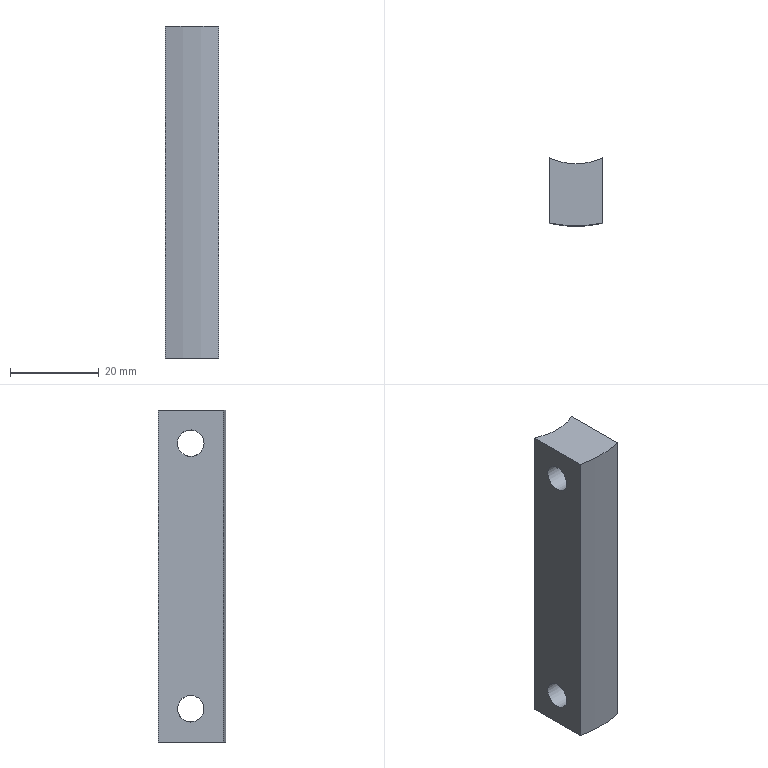Part | NX | features DATUM_CSYS 3, EXTRUDE 2, SKETCH 2 | 1 solid | 8 faces | box 12 x 15.351 x 75 mm | volume 12124 mm3 | plane 4 | cylinder 4 | commonest cylinder face diameters 6 x2 28 x1 56 x1
STEP:
#1=CARTESIAN_POINT('',(-6.,-20.,-27.));
#2=VERTEX_POINT('',#1);
#3=CARTESIAN_POINT('',(-6.,-20.,-30.));
#4=DIRECTION('',(-1.,0.,0.));
#5=DIRECTION('',(0.,0.,1.));
#6=AXIS2_PLACEMENT_3D('',#3,#4,#5);
#7=CIRCLE('',#6,3.);
#8=EDGE_CURVE('',#2,#2,#7,.T.);
#9=ORIENTED_EDGE('',*,*,#8,.F.);
#10=EDGE_LOOP('',(#9));
#11=FACE_BOUND('',#10,.T.);
#12=CARTESIAN_POINT('',(-6.,-20.,27.));
#13=VERTEX_POINT('',#12);
#14=CARTESIAN_POINT('',(-6.,-20.,30.));
#15=DIRECTION('',(-1.,0.,0.));
#16=DIRECTION('',(0.,0.,-1.));
#17=AXIS2_PLACEMENT_3D('',#14,#15,#16);
#18=CIRCLE('',#17,3.);
#19=EDGE_CURVE('',#13,#13,#18,.T.);
#20=ORIENTED_EDGE('',*,*,#19,.F.);
#21=EDGE_LOOP('',(#20));
#22=FACE_BOUND('',#21,.T.);
#23=CARTESIAN_POINT('',(-6.,-12.649,-37.5));
#24=VERTEX_POINT('',#23);
#25=CARTESIAN_POINT('',(-6.,-27.35,-37.5));
#26=VERTEX_POINT('',#25);
#27=CARTESIAN_POINT('',(-6.,-12.649,-37.5));
#28=DIRECTION('',(0.,-1.,0.));
#29=VECTOR('',#28,1000.);
#30=LINE('',#27,#29);
#31=EDGE_CURVE('',#24,#26,#30,.T.);
#32=ORIENTED_EDGE('',*,*,#31,.T.);
#33=CARTESIAN_POINT('',(-6.,-27.35,37.5));
#34=VERTEX_POINT('',#33);
#35=CARTESIAN_POINT('',(-6.,-27.35,37.5));
#36=DIRECTION('',(0.,0.,-1.));
#37=VECTOR('',#36,1000.);
#38=LINE('',#35,#37);
#39=EDGE_CURVE('',#34,#26,#38,.T.);
#40=ORIENTED_EDGE('',*,*,#39,.F.);
#41=CARTESIAN_POINT('',(-6.,-12.649,37.5));
#42=VERTEX_POINT('',#41);
#43=CARTESIAN_POINT('',(-6.,-12.649,37.5));
#44=DIRECTION('',(0.,-1.,0.));
#45=VECTOR('',#44,1000.);
#46=LINE('',#43,#45);
#47=EDGE_CURVE('',#42,#34,#46,.T.);
#48=ORIENTED_EDGE('',*,*,#47,.F.);
#49=CARTESIAN_POINT('',(-6.,-12.649,37.5));
#50=DIRECTION('',(0.,0.,-1.));
#51=VECTOR('',#50,1000.);
#52=LINE('',#49,#51);
#53=EDGE_CURVE('',#42,#24,#52,.T.);
#54=ORIENTED_EDGE('',*,*,#53,.T.);
#55=EDGE_LOOP('',(#32,#40,#48,#54));
#56=FACE_BOUND('',#55,.T.);
#57=CARTESIAN_POINT('',(-6.,-12.649,37.5));
#58=DIRECTION('',(1.,0.,0.));
#59=DIRECTION('',(0.,0.,-1.));
#60=AXIS2_PLACEMENT_3D('',#57,#58,#59);
#61=PLANE('',#60);
#62=ADVANCED_FACE('',(#11,#22,#56),#61,.F.);
#63=CARTESIAN_POINT('',(6.,-27.35,-37.5));
#64=VERTEX_POINT('',#63);
#65=CARTESIAN_POINT('',(-0.000002247,0.,-37.5));
#66=DIRECTION('',(0.,0.,1.));
#67=DIRECTION('',(1.,0.,0.));
#68=AXIS2_PLACEMENT_3D('',#65,#66,#67);
#69=CIRCLE('',#68,28.);
#70=EDGE_CURVE('',#26,#64,#69,.T.);
#71=ORIENTED_EDGE('',*,*,#70,.T.);
#72=CARTESIAN_POINT('',(6.,-27.35,37.5));
#73=VERTEX_POINT('',#72);
#74=CARTESIAN_POINT('',(6.,-27.35,37.5));
#75=DIRECTION('',(0.,0.,-1.));
#76=VECTOR('',#75,1000.);
#77=LINE('',#74,#76);
#78=EDGE_CURVE('',#73,#64,#77,.T.);
#79=ORIENTED_EDGE('',*,*,#78,.F.);
#80=CARTESIAN_POINT('',(-0.000002247,0.,37.5));
#81=DIRECTION('',(0.,0.,1.));
#82=DIRECTION('',(1.,0.,0.));
#83=AXIS2_PLACEMENT_3D('',#80,#81,#82);
#84=CIRCLE('',#83,28.);
#85=EDGE_CURVE('',#34,#73,#84,.T.);
#86=ORIENTED_EDGE('',*,*,#85,.F.);
#87=ORIENTED_EDGE('',*,*,#39,.T.);
#88=EDGE_LOOP('',(#71,#79,#86,#87));
#89=FACE_BOUND('',#88,.T.);
#90=CARTESIAN_POINT('',(-0.000002247,0.,37.5));
#91=DIRECTION('',(0.,0.,-1.));
#92=DIRECTION('',(-1.,0.,0.));
#93=AXIS2_PLACEMENT_3D('',#90,#91,#92);
#94=CYLINDRICAL_SURFACE('',#93,28.);
#95=ADVANCED_FACE('',(#89),#94,.T.);
#96=CARTESIAN_POINT('',(6.,-23.,-30.));
#97=VERTEX_POINT('',#96);
#98=CARTESIAN_POINT('',(6.,-20.,-30.));
#99=DIRECTION('',(-1.,0.,0.));
#100=DIRECTION('',(0.,-1.,0.));
#101=AXIS2_PLACEMENT_3D('',#98,#99,#100);
#102=CIRCLE('',#101,3.);
#103=EDGE_CURVE('',#97,#97,#102,.T.);
#104=ORIENTED_EDGE('',*,*,#103,.T.);
#105=EDGE_LOOP('',(#104));
#106=FACE_BOUND('',#105,.T.);
#107=CARTESIAN_POINT('',(6.,-23.,30.));
#108=VERTEX_POINT('',#107);
#109=CARTESIAN_POINT('',(6.,-20.,30.));
#110=DIRECTION('',(-1.,0.,0.));
#111=DIRECTION('',(0.,-1.,0.));
#112=AXIS2_PLACEMENT_3D('',#109,#110,#111);
#113=CIRCLE('',#112,3.);
#114=EDGE_CURVE('',#108,#108,#113,.T.);
#115=ORIENTED_EDGE('',*,*,#114,.T.);
#116=EDGE_LOOP('',(#115));
#117=FACE_BOUND('',#116,.T.);
#118=CARTESIAN_POINT('',(6.,-12.649,-37.5));
#119=VERTEX_POINT('',#118);
#120=CARTESIAN_POINT('',(6.,-27.35,-37.5));
#121=DIRECTION('',(0.,1.,0.));
#122=VECTOR('',#121,1000.);
#123=LINE('',#120,#122);
#124=EDGE_CURVE('',#64,#119,#123,.T.);
#125=ORIENTED_EDGE('',*,*,#124,.T.);
#126=CARTESIAN_POINT('',(6.,-12.649,37.5));
#127=VERTEX_POINT('',#126);
#128=CARTESIAN_POINT('',(6.,-12.649,37.5));
#129=DIRECTION('',(0.,0.,-1.));
#130=VECTOR('',#129,1000.);
#131=LINE('',#128,#130);
#132=EDGE_CURVE('',#127,#119,#131,.T.);
#133=ORIENTED_EDGE('',*,*,#132,.F.);
#134=CARTESIAN_POINT('',(6.,-27.35,37.5));
#135=DIRECTION('',(0.,1.,0.));
#136=VECTOR('',#135,1000.);
#137=LINE('',#134,#136);
#138=EDGE_CURVE('',#73,#127,#137,.T.);
#139=ORIENTED_EDGE('',*,*,#138,.F.);
#140=ORIENTED_EDGE('',*,*,#78,.T.);
#141=EDGE_LOOP('',(#125,#133,#139,#140));
#142=FACE_BOUND('',#141,.T.);
#143=CARTESIAN_POINT('',(6.,-27.35,37.5));
#144=DIRECTION('',(-1.,0.,0.));
#145=DIRECTION('',(0.,-1.,0.));
#146=AXIS2_PLACEMENT_3D('',#143,#144,#145);
#147=PLANE('',#146);
#148=ADVANCED_FACE('',(#106,#117,#142),#147,.F.);
#149=CARTESIAN_POINT('',(-0.000002247,0.,-37.5));
#150=DIRECTION('',(0.,0.,-1.));
#151=DIRECTION('',(1.,0.,0.));
#152=AXIS2_PLACEMENT_3D('',#149,#150,#151);
#153=CIRCLE('',#152,14.);
#154=EDGE_CURVE('',#119,#24,#153,.T.);
#155=ORIENTED_EDGE('',*,*,#154,.T.);
#156=ORIENTED_EDGE('',*,*,#53,.F.);
#157=CARTESIAN_POINT('',(-0.000002247,0.,37.5));
#158=DIRECTION('',(0.,0.,-1.));
#159=DIRECTION('',(1.,0.,0.));
#160=AXIS2_PLACEMENT_3D('',#157,#158,#159);
#161=CIRCLE('',#160,14.);
#162=EDGE_CURVE('',#127,#42,#161,.T.);
#163=ORIENTED_EDGE('',*,*,#162,.F.);
#164=ORIENTED_EDGE('',*,*,#132,.T.);
#165=EDGE_LOOP('',(#155,#156,#163,#164));
#166=FACE_BOUND('',#165,.T.);
#167=CARTESIAN_POINT('',(-0.000002247,0.,37.5));
#168=DIRECTION('',(0.,0.,-1.));
#169=DIRECTION('',(-1.,0.,0.));
#170=AXIS2_PLACEMENT_3D('',#167,#168,#169);
#171=CYLINDRICAL_SURFACE('',#170,14.);
#172=ADVANCED_FACE('',(#166),#171,.F.);
#173=ORIENTED_EDGE('',*,*,#47,.T.);
#174=ORIENTED_EDGE('',*,*,#85,.T.);
#175=ORIENTED_EDGE('',*,*,#138,.T.);
#176=ORIENTED_EDGE('',*,*,#162,.T.);
#177=EDGE_LOOP('',(#173,#174,#175,#176));
#178=FACE_BOUND('',#177,.T.);
#179=CARTESIAN_POINT('',(-0.000002247,0.,37.5));
#180=DIRECTION('',(0.,0.,1.));
#181=DIRECTION('',(1.,0.,0.));
#182=AXIS2_PLACEMENT_3D('',#179,#180,#181);
#183=PLANE('',#182);
#184=ADVANCED_FACE('',(#178),#183,.T.);
#185=ORIENTED_EDGE('',*,*,#31,.F.);
#186=ORIENTED_EDGE('',*,*,#154,.F.);
#187=ORIENTED_EDGE('',*,*,#124,.F.);
#188=ORIENTED_EDGE('',*,*,#70,.F.);
#189=EDGE_LOOP('',(#185,#186,#187,#188));
#190=FACE_BOUND('',#189,.T.);
#191=CARTESIAN_POINT('',(-0.000002247,0.,-37.5));
#192=DIRECTION('',(0.,0.,1.));
#193=DIRECTION('',(1.,0.,0.));
#194=AXIS2_PLACEMENT_3D('',#191,#192,#193);
#195=PLANE('',#194);
#196=ADVANCED_FACE('',(#190),#195,.F.);
#197=ORIENTED_EDGE('',*,*,#19,.T.);
#198=EDGE_LOOP('',(#197));
#199=FACE_BOUND('',#198,.T.);
#200=ORIENTED_EDGE('',*,*,#114,.F.);
#201=EDGE_LOOP('',(#200));
#202=FACE_BOUND('',#201,.T.);
#203=CARTESIAN_POINT('',(69.5,-20.,30.));
#204=DIRECTION('',(-1.,0.,0.));
#205=DIRECTION('',(0.,0.,1.));
#206=AXIS2_PLACEMENT_3D('',#203,#204,#205);
#207=CYLINDRICAL_SURFACE('',#206,3.);
#208=ADVANCED_FACE('',(#199,#202),#207,.F.);
#209=ORIENTED_EDGE('',*,*,#8,.T.);
#210=EDGE_LOOP('',(#209));
#211=FACE_BOUND('',#210,.T.);
#212=ORIENTED_EDGE('',*,*,#103,.F.);
#213=EDGE_LOOP('',(#212));
#214=FACE_BOUND('',#213,.T.);
#215=CARTESIAN_POINT('',(69.5,-20.,-30.));
#216=DIRECTION('',(-1.,0.,0.));
#217=DIRECTION('',(0.,0.,1.));
#218=AXIS2_PLACEMENT_3D('',#215,#216,#217);
#219=CYLINDRICAL_SURFACE('',#218,3.);
#220=ADVANCED_FACE('',(#211,#214),#219,.F.);
#221=CLOSED_SHELL('',(#62,#95,#148,#172,#184,#196,#208,#220));
#222=MANIFOLD_SOLID_BREP('',#221);
#223=(LENGTH_UNIT()NAMED_UNIT(*)SI_UNIT(.MILLI.,.METRE.));
#224=UNCERTAINTY_MEASURE_WITH_UNIT(LENGTH_MEASURE(0.00001),#223,'','');
#225=(NAMED_UNIT(*)PLANE_ANGLE_UNIT()SI_UNIT($,.RADIAN.));
#226=(NAMED_UNIT(*)SI_UNIT($,.STERADIAN.)SOLID_ANGLE_UNIT());
#227=(GEOMETRIC_REPRESENTATION_CONTEXT(3)GLOBAL_UNCERTAINTY_ASSIGNED_CONTEXT((#224))GLOBAL_UNIT_ASSIGNED_CONTEXT((#223,#225,#226))REPRESENTATION_CONTEXT('',''));
#228=ADVANCED_BREP_SHAPE_REPRESENTATION('',(#222),#227);